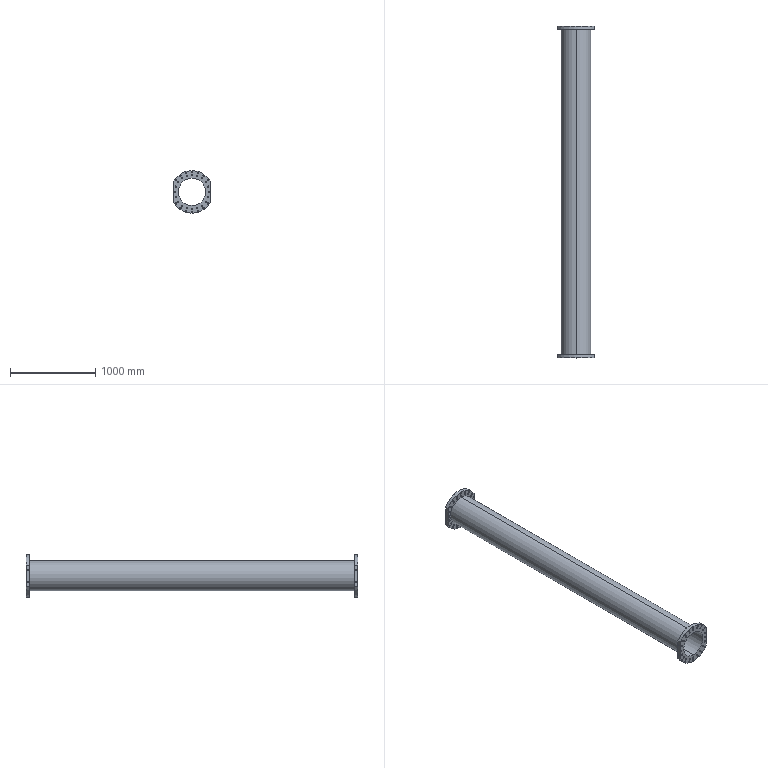Part | SolidWorks | features Extrusion 1, HoleWzd 1, ICE 1, LPattern 1 | 1 solid | 170 faces | box 430 x 3897 x 500 mm | volume 70114702 mm3 | cylinder 154 | plane 16 | commonest cylinder face diameters 16 x144 500 x6 320 x2 351 x2